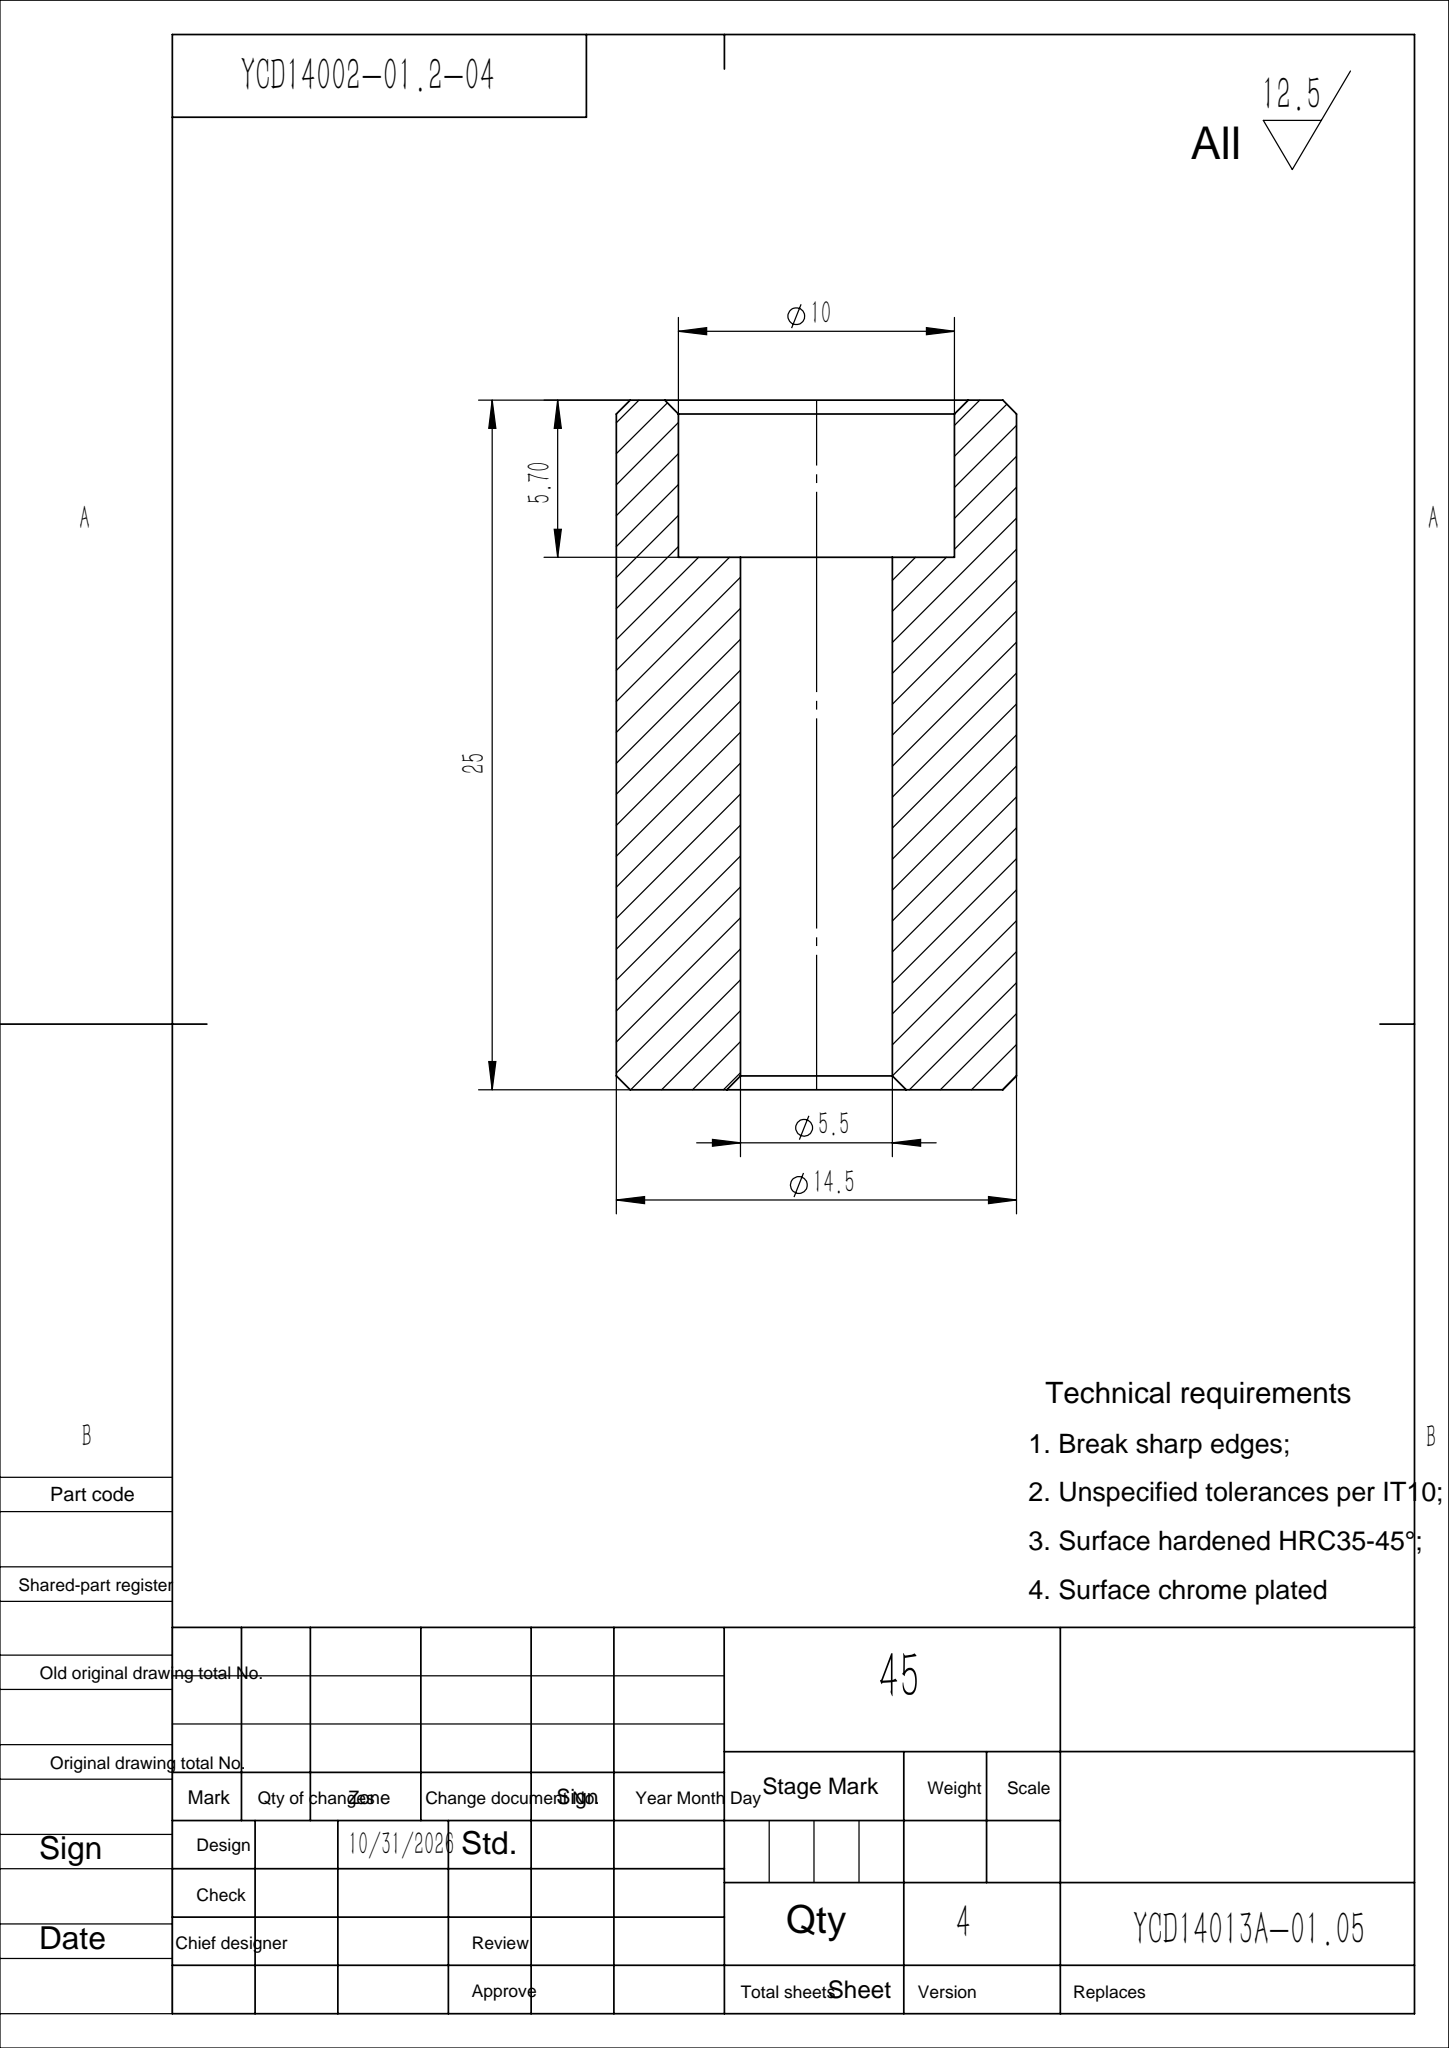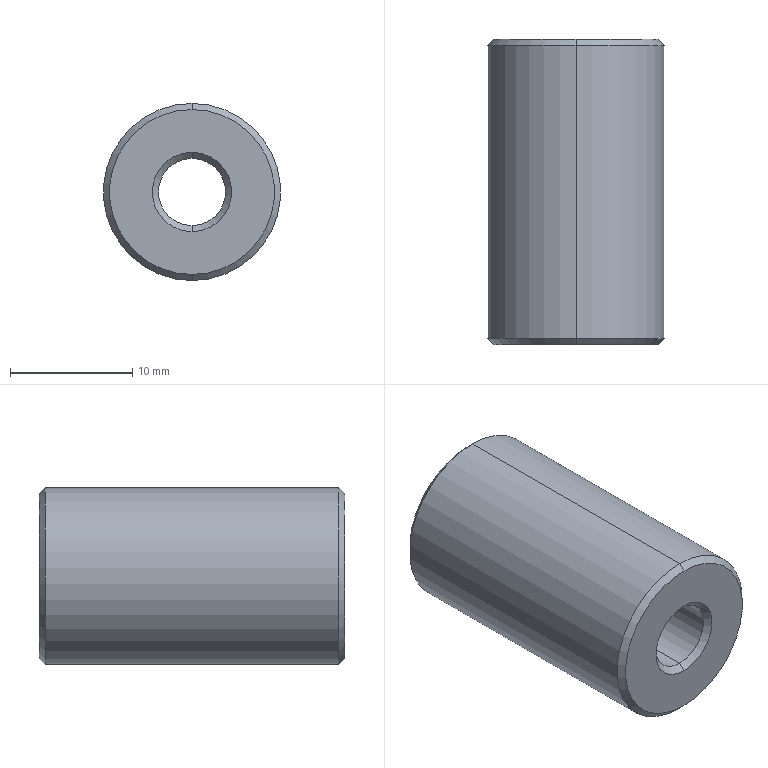Part | SolidWorks | features Chamfer 1, Extrusion 1, HoleWzd 1 | 1 solid | 17 faces | box 14.5 x 25 x 14.5 mm | volume 3205 mm3 | cone 8 | cylinder 6 | plane 3 | commonest cylinder face diameters 5.5 x2 10 x2 14.5 x2
STEP:
#1=CARTESIAN_POINT('',(0.,0.5,2.75));
#2=VERTEX_POINT('',#1);
#3=CARTESIAN_POINT('',(0.,0.5,-2.75));
#4=VERTEX_POINT('',#3);
#5=CARTESIAN_POINT('',(0.,0.5,0.));
#6=DIRECTION('',(0.,-1.,0.));
#7=DIRECTION('',(0.,0.,1.));
#8=AXIS2_PLACEMENT_3D('',#5,#6,#7);
#9=CIRCLE('',#8,2.75);
#10=EDGE_CURVE('',#2,#4,#9,.T.);
#11=ORIENTED_EDGE('',*,*,#10,.F.);
#12=CARTESIAN_POINT('',(0.,0.,3.25));
#13=VERTEX_POINT('',#12);
#14=CARTESIAN_POINT('',(0.,0.,3.25));
#15=DIRECTION('',(0.,-0.7071,0.7071));
#16=VECTOR('',#15,1000.);
#17=LINE('',#14,#16);
#18=EDGE_CURVE('',#2,#13,#17,.T.);
#19=ORIENTED_EDGE('',*,*,#18,.T.);
#20=CARTESIAN_POINT('',(0.,0.,-3.25));
#21=VERTEX_POINT('',#20);
#22=CARTESIAN_POINT('',(0.,0.,0.));
#23=DIRECTION('',(0.,1.,0.));
#24=DIRECTION('',(0.,0.,1.));
#25=AXIS2_PLACEMENT_3D('',#22,#23,#24);
#26=CIRCLE('',#25,3.25);
#27=EDGE_CURVE('',#21,#13,#26,.T.);
#28=ORIENTED_EDGE('',*,*,#27,.F.);
#29=CARTESIAN_POINT('',(0.,0.,-3.25));
#30=DIRECTION('',(0.,-0.7071,-0.7071));
#31=VECTOR('',#30,1000.);
#32=LINE('',#29,#31);
#33=EDGE_CURVE('',#4,#21,#32,.T.);
#34=ORIENTED_EDGE('',*,*,#33,.F.);
#35=EDGE_LOOP('',(#11,#19,#28,#34));
#36=FACE_OUTER_BOUND('',#35,.T.);
#37=CARTESIAN_POINT('',(0.,0.,0.));
#38=DIRECTION('',(0.,-1.,0.));
#39=DIRECTION('',(0.,0.,-1.));
#40=AXIS2_PLACEMENT_3D('',#37,#38,#39);
#41=CONICAL_SURFACE('',#40,3.25,0.7854);
#42=ADVANCED_FACE('',(#36),#41,.F.);
#43=CARTESIAN_POINT('',(0.,0.,-6.75));
#44=VERTEX_POINT('',#43);
#45=CARTESIAN_POINT('',(0.,0.,6.75));
#46=VERTEX_POINT('',#45);
#47=CARTESIAN_POINT('',(0.,0.,0.));
#48=DIRECTION('',(0.,-1.,0.));
#49=DIRECTION('',(0.,0.,1.));
#50=AXIS2_PLACEMENT_3D('',#47,#48,#49);
#51=CIRCLE('',#50,6.75);
#52=EDGE_CURVE('',#44,#46,#51,.T.);
#53=ORIENTED_EDGE('',*,*,#52,.F.);
#54=CARTESIAN_POINT('',(0.,0.5,-7.25));
#55=VERTEX_POINT('',#54);
#56=CARTESIAN_POINT('',(0.,0.5,-7.25));
#57=DIRECTION('',(0.,0.7071,-0.7071));
#58=VECTOR('',#57,1000.);
#59=LINE('',#56,#58);
#60=EDGE_CURVE('',#44,#55,#59,.T.);
#61=ORIENTED_EDGE('',*,*,#60,.T.);
#62=CARTESIAN_POINT('',(0.,0.5,7.25));
#63=VERTEX_POINT('',#62);
#64=CARTESIAN_POINT('',(0.,0.5,0.));
#65=DIRECTION('',(0.,1.,0.));
#66=DIRECTION('',(0.,0.,1.));
#67=AXIS2_PLACEMENT_3D('',#64,#65,#66);
#68=CIRCLE('',#67,7.25);
#69=EDGE_CURVE('',#63,#55,#68,.T.);
#70=ORIENTED_EDGE('',*,*,#69,.F.);
#71=CARTESIAN_POINT('',(0.,0.5,7.25));
#72=DIRECTION('',(0.,0.7071,0.7071));
#73=VECTOR('',#72,1000.);
#74=LINE('',#71,#73);
#75=EDGE_CURVE('',#46,#63,#74,.T.);
#76=ORIENTED_EDGE('',*,*,#75,.F.);
#77=EDGE_LOOP('',(#53,#61,#70,#76));
#78=FACE_OUTER_BOUND('',#77,.T.);
#79=CARTESIAN_POINT('',(0.,0.5,0.));
#80=DIRECTION('',(0.,1.,0.));
#81=DIRECTION('',(0.,0.,1.));
#82=AXIS2_PLACEMENT_3D('',#79,#80,#81);
#83=CONICAL_SURFACE('',#82,7.25,0.7854);
#84=ADVANCED_FACE('',(#78),#83,.T.);
#85=CARTESIAN_POINT('',(0.,24.5,-5.));
#86=VERTEX_POINT('',#85);
#87=CARTESIAN_POINT('',(0.,24.5,5.));
#88=VERTEX_POINT('',#87);
#89=CARTESIAN_POINT('',(0.,24.5,0.));
#90=DIRECTION('',(0.,1.,0.));
#91=DIRECTION('',(0.,0.,1.));
#92=AXIS2_PLACEMENT_3D('',#89,#90,#91);
#93=CIRCLE('',#92,5.);
#94=EDGE_CURVE('',#86,#88,#93,.T.);
#95=ORIENTED_EDGE('',*,*,#94,.F.);
#96=CARTESIAN_POINT('',(0.,25.,-5.5));
#97=VERTEX_POINT('',#96);
#98=CARTESIAN_POINT('',(0.,24.5,-5.));
#99=DIRECTION('',(0.,0.7071,-0.7071));
#100=VECTOR('',#99,1000.);
#101=LINE('',#98,#100);
#102=EDGE_CURVE('',#86,#97,#101,.T.);
#103=ORIENTED_EDGE('',*,*,#102,.T.);
#104=CARTESIAN_POINT('',(0.,25.,5.5));
#105=VERTEX_POINT('',#104);
#106=CARTESIAN_POINT('',(0.,25.,0.));
#107=DIRECTION('',(0.,-1.,0.));
#108=DIRECTION('',(0.,0.,1.));
#109=AXIS2_PLACEMENT_3D('',#106,#107,#108);
#110=CIRCLE('',#109,5.5);
#111=EDGE_CURVE('',#105,#97,#110,.T.);
#112=ORIENTED_EDGE('',*,*,#111,.F.);
#113=CARTESIAN_POINT('',(0.,24.5,5.));
#114=DIRECTION('',(0.,0.7071,0.7071));
#115=VECTOR('',#114,1000.);
#116=LINE('',#113,#115);
#117=EDGE_CURVE('',#88,#105,#116,.T.);
#118=ORIENTED_EDGE('',*,*,#117,.F.);
#119=EDGE_LOOP('',(#95,#103,#112,#118));
#120=FACE_OUTER_BOUND('',#119,.T.);
#121=CARTESIAN_POINT('',(0.,24.5,0.));
#122=DIRECTION('',(0.,1.,0.));
#123=DIRECTION('',(0.,0.,1.));
#124=AXIS2_PLACEMENT_3D('',#121,#122,#123);
#125=CONICAL_SURFACE('',#124,5.,0.7854);
#126=ADVANCED_FACE('',(#120),#125,.F.);
#127=CARTESIAN_POINT('',(0.,25.,6.75));
#128=VERTEX_POINT('',#127);
#129=CARTESIAN_POINT('',(0.,25.,-6.75));
#130=VERTEX_POINT('',#129);
#131=CARTESIAN_POINT('',(0.,25.,0.));
#132=DIRECTION('',(0.,1.,0.));
#133=DIRECTION('',(0.,0.,1.));
#134=AXIS2_PLACEMENT_3D('',#131,#132,#133);
#135=CIRCLE('',#134,6.75);
#136=EDGE_CURVE('',#128,#130,#135,.T.);
#137=ORIENTED_EDGE('',*,*,#136,.F.);
#138=CARTESIAN_POINT('',(0.,24.5,7.25));
#139=VERTEX_POINT('',#138);
#140=CARTESIAN_POINT('',(0.,25.,6.75));
#141=DIRECTION('',(0.,-0.7071,0.7071));
#142=VECTOR('',#141,1000.);
#143=LINE('',#140,#142);
#144=EDGE_CURVE('',#128,#139,#143,.T.);
#145=ORIENTED_EDGE('',*,*,#144,.T.);
#146=CARTESIAN_POINT('',(0.,24.5,-7.25));
#147=VERTEX_POINT('',#146);
#148=CARTESIAN_POINT('',(0.,24.5,0.));
#149=DIRECTION('',(0.,-1.,0.));
#150=DIRECTION('',(0.,0.,1.));
#151=AXIS2_PLACEMENT_3D('',#148,#149,#150);
#152=CIRCLE('',#151,7.25);
#153=EDGE_CURVE('',#147,#139,#152,.T.);
#154=ORIENTED_EDGE('',*,*,#153,.F.);
#155=CARTESIAN_POINT('',(0.,25.,-6.75));
#156=DIRECTION('',(0.,-0.7071,-0.7071));
#157=VECTOR('',#156,1000.);
#158=LINE('',#155,#157);
#159=EDGE_CURVE('',#130,#147,#158,.T.);
#160=ORIENTED_EDGE('',*,*,#159,.F.);
#161=EDGE_LOOP('',(#137,#145,#154,#160));
#162=FACE_OUTER_BOUND('',#161,.T.);
#163=CARTESIAN_POINT('',(0.,25.,0.));
#164=DIRECTION('',(0.,-1.,0.));
#165=DIRECTION('',(0.,0.,-1.));
#166=AXIS2_PLACEMENT_3D('',#163,#164,#165);
#167=CONICAL_SURFACE('',#166,6.75,0.7854);
#168=ADVANCED_FACE('',(#162),#167,.T.);
#169=CARTESIAN_POINT('',(0.,19.3,-5.));
#170=VERTEX_POINT('',#169);
#171=CARTESIAN_POINT('',(0.,19.3,5.));
#172=VERTEX_POINT('',#171);
#173=CARTESIAN_POINT('',(0.,19.3,0.));
#174=DIRECTION('',(0.,1.,0.));
#175=DIRECTION('',(0.,0.,1.));
#176=AXIS2_PLACEMENT_3D('',#173,#174,#175);
#177=CIRCLE('',#176,5.);
#178=EDGE_CURVE('',#170,#172,#177,.T.);
#179=ORIENTED_EDGE('',*,*,#178,.F.);
#180=CARTESIAN_POINT('',(0.,25.,-5.));
#181=DIRECTION('',(0.,1.,0.));
#182=VECTOR('',#181,1000.);
#183=LINE('',#180,#182);
#184=EDGE_CURVE('',#170,#86,#183,.T.);
#185=ORIENTED_EDGE('',*,*,#184,.T.);
#186=ORIENTED_EDGE('',*,*,#94,.T.);
#187=CARTESIAN_POINT('',(0.,25.,5.));
#188=DIRECTION('',(0.,1.,0.));
#189=VECTOR('',#188,1000.);
#190=LINE('',#187,#189);
#191=EDGE_CURVE('',#172,#88,#190,.T.);
#192=ORIENTED_EDGE('',*,*,#191,.F.);
#193=EDGE_LOOP('',(#179,#185,#186,#192));
#194=FACE_OUTER_BOUND('',#193,.T.);
#195=CARTESIAN_POINT('',(0.,25.,0.));
#196=DIRECTION('',(0.,1.,0.));
#197=DIRECTION('',(0.,0.,1.));
#198=AXIS2_PLACEMENT_3D('',#195,#196,#197);
#199=CYLINDRICAL_SURFACE('',#198,5.);
#200=ADVANCED_FACE('',(#194),#199,.F.);
#201=ORIENTED_EDGE('',*,*,#10,.T.);
#202=CARTESIAN_POINT('',(0.,19.3,-2.75));
#203=VERTEX_POINT('',#202);
#204=CARTESIAN_POINT('',(0.,25.,-2.75));
#205=DIRECTION('',(0.,1.,0.));
#206=VECTOR('',#205,1000.);
#207=LINE('',#204,#206);
#208=EDGE_CURVE('',#4,#203,#207,.T.);
#209=ORIENTED_EDGE('',*,*,#208,.T.);
#210=CARTESIAN_POINT('',(0.,19.3,2.75));
#211=VERTEX_POINT('',#210);
#212=CARTESIAN_POINT('',(0.,19.3,0.));
#213=DIRECTION('',(0.,1.,0.));
#214=DIRECTION('',(0.,0.,1.));
#215=AXIS2_PLACEMENT_3D('',#212,#213,#214);
#216=CIRCLE('',#215,2.75);
#217=EDGE_CURVE('',#203,#211,#216,.T.);
#218=ORIENTED_EDGE('',*,*,#217,.T.);
#219=CARTESIAN_POINT('',(0.,25.,2.75));
#220=DIRECTION('',(0.,1.,0.));
#221=VECTOR('',#220,1000.);
#222=LINE('',#219,#221);
#223=EDGE_CURVE('',#2,#211,#222,.T.);
#224=ORIENTED_EDGE('',*,*,#223,.F.);
#225=EDGE_LOOP('',(#201,#209,#218,#224));
#226=FACE_OUTER_BOUND('',#225,.T.);
#227=CARTESIAN_POINT('',(0.,25.,0.));
#228=DIRECTION('',(0.,1.,0.));
#229=DIRECTION('',(0.,0.,1.));
#230=AXIS2_PLACEMENT_3D('',#227,#228,#229);
#231=CYLINDRICAL_SURFACE('',#230,2.75);
#232=ADVANCED_FACE('',(#226),#231,.F.);
#233=ORIENTED_EDGE('',*,*,#153,.T.);
#234=CARTESIAN_POINT('',(0.,25.,7.25));
#235=DIRECTION('',(0.,-1.,0.));
#236=VECTOR('',#235,1000.);
#237=LINE('',#234,#236);
#238=EDGE_CURVE('',#139,#63,#237,.T.);
#239=ORIENTED_EDGE('',*,*,#238,.T.);
#240=ORIENTED_EDGE('',*,*,#69,.T.);
#241=CARTESIAN_POINT('',(0.,25.,-7.25));
#242=DIRECTION('',(0.,-1.,0.));
#243=VECTOR('',#242,1000.);
#244=LINE('',#241,#243);
#245=EDGE_CURVE('',#147,#55,#244,.T.);
#246=ORIENTED_EDGE('',*,*,#245,.F.);
#247=EDGE_LOOP('',(#233,#239,#240,#246));
#248=FACE_OUTER_BOUND('',#247,.T.);
#249=CARTESIAN_POINT('',(0.,25.,0.));
#250=DIRECTION('',(0.,-1.,0.));
#251=DIRECTION('',(0.,0.,-1.));
#252=AXIS2_PLACEMENT_3D('',#249,#250,#251);
#253=CYLINDRICAL_SURFACE('',#252,7.25);
#254=ADVANCED_FACE('',(#248),#253,.T.);
#255=ORIENTED_EDGE('',*,*,#238,.F.);
#256=CARTESIAN_POINT('',(0.,24.5,0.));
#257=DIRECTION('',(0.,-1.,0.));
#258=DIRECTION('',(0.,0.,1.));
#259=AXIS2_PLACEMENT_3D('',#256,#257,#258);
#260=CIRCLE('',#259,7.25);
#261=EDGE_CURVE('',#139,#147,#260,.T.);
#262=ORIENTED_EDGE('',*,*,#261,.T.);
#263=ORIENTED_EDGE('',*,*,#245,.T.);
#264=CARTESIAN_POINT('',(0.,0.5,0.));
#265=DIRECTION('',(0.,1.,0.));
#266=DIRECTION('',(0.,0.,1.));
#267=AXIS2_PLACEMENT_3D('',#264,#265,#266);
#268=CIRCLE('',#267,7.25);
#269=EDGE_CURVE('',#55,#63,#268,.T.);
#270=ORIENTED_EDGE('',*,*,#269,.T.);
#271=EDGE_LOOP('',(#255,#262,#263,#270));
#272=FACE_OUTER_BOUND('',#271,.T.);
#273=CARTESIAN_POINT('',(0.,25.,0.));
#274=DIRECTION('',(0.,-1.,0.));
#275=DIRECTION('',(0.,0.,-1.));
#276=AXIS2_PLACEMENT_3D('',#273,#274,#275);
#277=CYLINDRICAL_SURFACE('',#276,7.25);
#278=ADVANCED_FACE('',(#272),#277,.T.);
#279=CARTESIAN_POINT('',(0.,25.,0.));
#280=DIRECTION('',(0.,1.,0.));
#281=DIRECTION('',(0.,0.,1.));
#282=AXIS2_PLACEMENT_3D('',#279,#280,#281);
#283=CIRCLE('',#282,6.75);
#284=EDGE_CURVE('',#130,#128,#283,.T.);
#285=ORIENTED_EDGE('',*,*,#284,.T.);
#286=ORIENTED_EDGE('',*,*,#136,.T.);
#287=EDGE_LOOP('',(#285,#286));
#288=FACE_OUTER_BOUND('',#287,.T.);
#289=ORIENTED_EDGE('',*,*,#111,.T.);
#290=CARTESIAN_POINT('',(0.,25.,0.));
#291=DIRECTION('',(0.,-1.,0.));
#292=DIRECTION('',(0.,0.,1.));
#293=AXIS2_PLACEMENT_3D('',#290,#291,#292);
#294=CIRCLE('',#293,5.5);
#295=EDGE_CURVE('',#97,#105,#294,.T.);
#296=ORIENTED_EDGE('',*,*,#295,.T.);
#297=EDGE_LOOP('',(#289,#296));
#298=FACE_BOUND('',#297,.T.);
#299=CARTESIAN_POINT('',(0.,25.,0.));
#300=DIRECTION('',(0.,1.,0.));
#301=DIRECTION('',(0.,0.,1.));
#302=AXIS2_PLACEMENT_3D('',#299,#300,#301);
#303=PLANE('',#302);
#304=ADVANCED_FACE('',(#288,#298),#303,.T.);
#305=CARTESIAN_POINT('',(0.,0.,0.));
#306=DIRECTION('',(0.,-1.,0.));
#307=DIRECTION('',(0.,0.,1.));
#308=AXIS2_PLACEMENT_3D('',#305,#306,#307);
#309=CIRCLE('',#308,6.75);
#310=EDGE_CURVE('',#46,#44,#309,.T.);
#311=ORIENTED_EDGE('',*,*,#310,.T.);
#312=ORIENTED_EDGE('',*,*,#52,.T.);
#313=EDGE_LOOP('',(#311,#312));
#314=FACE_OUTER_BOUND('',#313,.T.);
#315=ORIENTED_EDGE('',*,*,#27,.T.);
#316=CARTESIAN_POINT('',(0.,0.,0.));
#317=DIRECTION('',(0.,1.,0.));
#318=DIRECTION('',(0.,0.,1.));
#319=AXIS2_PLACEMENT_3D('',#316,#317,#318);
#320=CIRCLE('',#319,3.25);
#321=EDGE_CURVE('',#13,#21,#320,.T.);
#322=ORIENTED_EDGE('',*,*,#321,.T.);
#323=EDGE_LOOP('',(#315,#322));
#324=FACE_BOUND('',#323,.T.);
#325=CARTESIAN_POINT('',(0.,0.,0.));
#326=DIRECTION('',(0.,1.,0.));
#327=DIRECTION('',(0.,0.,1.));
#328=AXIS2_PLACEMENT_3D('',#325,#326,#327);
#329=PLANE('',#328);
#330=ADVANCED_FACE('',(#314,#324),#329,.F.);
#331=ORIENTED_EDGE('',*,*,#208,.F.);
#332=CARTESIAN_POINT('',(0.,0.5,0.));
#333=DIRECTION('',(0.,-1.,0.));
#334=DIRECTION('',(0.,0.,1.));
#335=AXIS2_PLACEMENT_3D('',#332,#333,#334);
#336=CIRCLE('',#335,2.75);
#337=EDGE_CURVE('',#4,#2,#336,.T.);
#338=ORIENTED_EDGE('',*,*,#337,.T.);
#339=ORIENTED_EDGE('',*,*,#223,.T.);
#340=CARTESIAN_POINT('',(0.,19.3,0.));
#341=DIRECTION('',(0.,1.,0.));
#342=DIRECTION('',(0.,0.,1.));
#343=AXIS2_PLACEMENT_3D('',#340,#341,#342);
#344=CIRCLE('',#343,2.75);
#345=EDGE_CURVE('',#211,#203,#344,.T.);
#346=ORIENTED_EDGE('',*,*,#345,.T.);
#347=EDGE_LOOP('',(#331,#338,#339,#346));
#348=FACE_OUTER_BOUND('',#347,.T.);
#349=CARTESIAN_POINT('',(0.,25.,0.));
#350=DIRECTION('',(0.,1.,0.));
#351=DIRECTION('',(0.,0.,1.));
#352=AXIS2_PLACEMENT_3D('',#349,#350,#351);
#353=CYLINDRICAL_SURFACE('',#352,2.75);
#354=ADVANCED_FACE('',(#348),#353,.F.);
#355=ORIENTED_EDGE('',*,*,#345,.F.);
#356=ORIENTED_EDGE('',*,*,#217,.F.);
#357=EDGE_LOOP('',(#355,#356));
#358=FACE_BOUND('',#357,.T.);
#359=CARTESIAN_POINT('',(0.,19.3,0.));
#360=DIRECTION('',(0.,1.,0.));
#361=DIRECTION('',(0.,0.,1.));
#362=AXIS2_PLACEMENT_3D('',#359,#360,#361);
#363=CIRCLE('',#362,5.);
#364=EDGE_CURVE('',#172,#170,#363,.T.);
#365=ORIENTED_EDGE('',*,*,#364,.T.);
#366=ORIENTED_EDGE('',*,*,#178,.T.);
#367=EDGE_LOOP('',(#365,#366));
#368=FACE_OUTER_BOUND('',#367,.T.);
#369=CARTESIAN_POINT('',(2.75,19.3,0.));
#370=DIRECTION('',(0.,-1.,0.));
#371=DIRECTION('',(0.,0.,-1.));
#372=AXIS2_PLACEMENT_3D('',#369,#370,#371);
#373=PLANE('',#372);
#374=ADVANCED_FACE('',(#358,#368),#373,.F.);
#375=ORIENTED_EDGE('',*,*,#184,.F.);
#376=ORIENTED_EDGE('',*,*,#364,.F.);
#377=ORIENTED_EDGE('',*,*,#191,.T.);
#378=CARTESIAN_POINT('',(0.,24.5,0.));
#379=DIRECTION('',(0.,1.,0.));
#380=DIRECTION('',(0.,0.,1.));
#381=AXIS2_PLACEMENT_3D('',#378,#379,#380);
#382=CIRCLE('',#381,5.);
#383=EDGE_CURVE('',#88,#86,#382,.T.);
#384=ORIENTED_EDGE('',*,*,#383,.T.);
#385=EDGE_LOOP('',(#375,#376,#377,#384));
#386=FACE_OUTER_BOUND('',#385,.T.);
#387=CARTESIAN_POINT('',(0.,25.,0.));
#388=DIRECTION('',(0.,1.,0.));
#389=DIRECTION('',(0.,0.,1.));
#390=AXIS2_PLACEMENT_3D('',#387,#388,#389);
#391=CYLINDRICAL_SURFACE('',#390,5.);
#392=ADVANCED_FACE('',(#386),#391,.F.);
#393=ORIENTED_EDGE('',*,*,#144,.F.);
#394=ORIENTED_EDGE('',*,*,#284,.F.);
#395=ORIENTED_EDGE('',*,*,#159,.T.);
#396=ORIENTED_EDGE('',*,*,#261,.F.);
#397=EDGE_LOOP('',(#393,#394,#395,#396));
#398=FACE_OUTER_BOUND('',#397,.T.);
#399=CARTESIAN_POINT('',(0.,25.,0.));
#400=DIRECTION('',(0.,-1.,0.));
#401=DIRECTION('',(0.,0.,-1.));
#402=AXIS2_PLACEMENT_3D('',#399,#400,#401);
#403=CONICAL_SURFACE('',#402,6.75,0.7854);
#404=ADVANCED_FACE('',(#398),#403,.T.);
#405=ORIENTED_EDGE('',*,*,#102,.F.);
#406=ORIENTED_EDGE('',*,*,#383,.F.);
#407=ORIENTED_EDGE('',*,*,#117,.T.);
#408=ORIENTED_EDGE('',*,*,#295,.F.);
#409=EDGE_LOOP('',(#405,#406,#407,#408));
#410=FACE_OUTER_BOUND('',#409,.T.);
#411=CARTESIAN_POINT('',(0.,24.5,0.));
#412=DIRECTION('',(0.,1.,0.));
#413=DIRECTION('',(0.,0.,1.));
#414=AXIS2_PLACEMENT_3D('',#411,#412,#413);
#415=CONICAL_SURFACE('',#414,5.,0.7854);
#416=ADVANCED_FACE('',(#410),#415,.F.);
#417=ORIENTED_EDGE('',*,*,#60,.F.);
#418=ORIENTED_EDGE('',*,*,#310,.F.);
#419=ORIENTED_EDGE('',*,*,#75,.T.);
#420=ORIENTED_EDGE('',*,*,#269,.F.);
#421=EDGE_LOOP('',(#417,#418,#419,#420));
#422=FACE_OUTER_BOUND('',#421,.T.);
#423=CARTESIAN_POINT('',(0.,0.5,0.));
#424=DIRECTION('',(0.,1.,0.));
#425=DIRECTION('',(0.,0.,1.));
#426=AXIS2_PLACEMENT_3D('',#423,#424,#425);
#427=CONICAL_SURFACE('',#426,7.25,0.7854);
#428=ADVANCED_FACE('',(#422),#427,.T.);
#429=ORIENTED_EDGE('',*,*,#18,.F.);
#430=ORIENTED_EDGE('',*,*,#337,.F.);
#431=ORIENTED_EDGE('',*,*,#33,.T.);
#432=ORIENTED_EDGE('',*,*,#321,.F.);
#433=EDGE_LOOP('',(#429,#430,#431,#432));
#434=FACE_OUTER_BOUND('',#433,.T.);
#435=CARTESIAN_POINT('',(0.,0.,0.));
#436=DIRECTION('',(0.,-1.,0.));
#437=DIRECTION('',(0.,0.,-1.));
#438=AXIS2_PLACEMENT_3D('',#435,#436,#437);
#439=CONICAL_SURFACE('',#438,3.25,0.7854);
#440=ADVANCED_FACE('',(#434),#439,.F.);
#441=CLOSED_SHELL('',(#42,#84,#126,#168,#200,#232,#254,#278,#304,#330,#354,#374,#392,#404,#416,#428,#440));
#442=MANIFOLD_SOLID_BREP('',#441);
#443=CARTESIAN_POINT('',(0.,0.,0.));
#444=DIRECTION('',(0.,0.,1.));
#445=DIRECTION('',(1.,0.,0.));
#446=AXIS2_PLACEMENT_3D('',#443,#444,#445);
#447=(LENGTH_UNIT()NAMED_UNIT(*)SI_UNIT(.MILLI.,.METRE.));
#448=UNCERTAINTY_MEASURE_WITH_UNIT(LENGTH_MEASURE(0.00001),#447,'','');
#449=(NAMED_UNIT(*)PLANE_ANGLE_UNIT()SI_UNIT($,.RADIAN.));
#450=(NAMED_UNIT(*)SI_UNIT($,.STERADIAN.)SOLID_ANGLE_UNIT());
#451=(GEOMETRIC_REPRESENTATION_CONTEXT(3)GLOBAL_UNCERTAINTY_ASSIGNED_CONTEXT((#448))GLOBAL_UNIT_ASSIGNED_CONTEXT((#447,#449,#450))REPRESENTATION_CONTEXT('',''));
#452=ADVANCED_BREP_SHAPE_REPRESENTATION('',(#442,#446),#451);